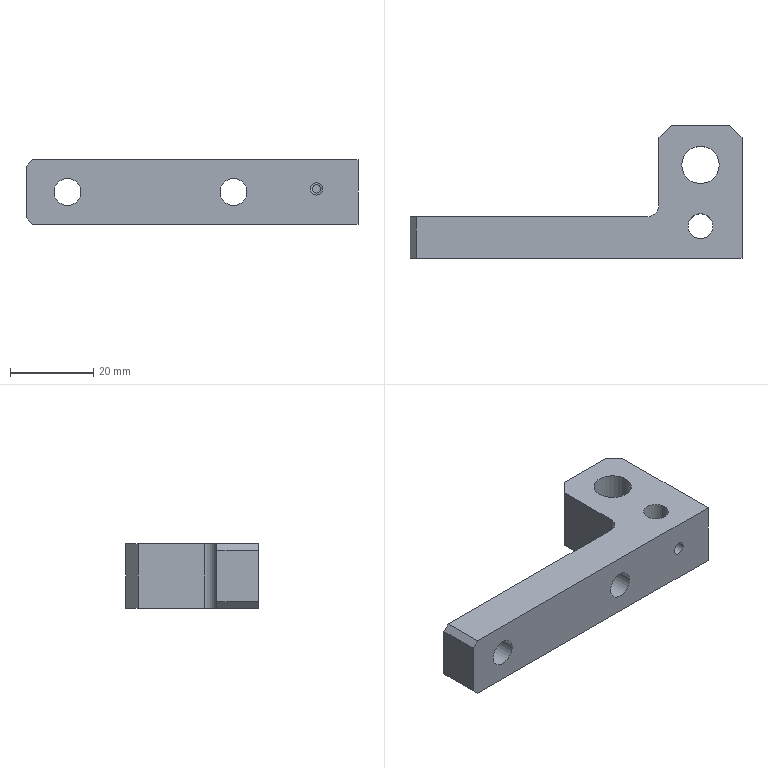NC program | NX | posted with a generic post | part box 80 x 32 x 15.5 mm
Lines 1772 to 1848 of 1848:
(PLANAR_MILL_3 , TOOL : D63面刀)
N3542 T10 M6
N3544 G54
N3546 G17 G0 G90 X74.5 Y2.5 B0. C0. S1600 M3
N3548 G43 Z20. H10
N3550 Z3.
N3552 G94 G1 Z0. F600.
N3554 X40.
N3556 X-40.
N3558 X-74.5
N3560 Z3.
N3562 G0 Z20.
N3564 M5
(PLANAR_MILL_6 , TOOL : 倒角D4-90度)
N3566 T05 M6
N3568 G54
N3570 G17 G0 G90 X-40. Y19.5 B0. C0. S3000 M3
N3572 G43 Z20. H5
N3574 Z1.5
N3576 G94 G1 Z-1.5 F800.
N3578 G41 Y17.5 D5
N3580 X40.
N3582 G2 X41.5 Y16. R1.5
N3584 G1 Y6.
N3586 G2 X40. Y4.5 R1.5
N3588 G1 X-17.
N3590 G3 X-18.5 Y3. R1.5
N3592 G1 Y-13.
N3594 G2 X-18.939 Y-14.061 R1.5
N3596 G1 X-21.939 Y-17.061
N3598 G2 X-23. Y-17.5 R1.5
N3600 G1 X-37.
N3602 G2 X-38.061 Y-17.061 R1.5
N3604 G1 X-41.061 Y-14.061
N3606 G2 X-41.5 Y-13. R1.5
N3608 G1 Y16.
N3610 G2 X-40. Y17.5 R1.5
N3612 G40
N3614 G1 Y19.5
N3616 Z1.5
N3618 G0 Z20.
(PLANAR_MILL_6_COPY_1 , TOOL : 倒角D4-90度)
N3620 X-30.119 Y7.924
N3622 Z0.5
N3624 G1 Z-1.5
N3626 G41 X-29.134 Y7.75
N3628 X-29.
N3630 G3 X-28.5 Y8.25 R0.5
N3632 X-30. Y9.75 R1.5
N3634 X-28.5 Y8.25 R-1.5
N3636 X-29. Y8.75 R0.5
N3638 G1 X-29.134
N3640 G40
N3642 X-30.119 Y8.576
N3644 Z0.5
N3646 G0 Z20.
N3648 X-28.535 Y-6.826
N3650 Z0.5
N3652 G1 Z-1.5
N3654 G41 X-27.551 Y-7.
N3656 X-27.5
N3658 G3 X-27. Y-6.5 R0.5
N3660 X-30. Y-3.5 R3.
N3662 X-27. Y-6.5 R-3.
N3664 X-27.551 Y-6. R0.503
N3666 G40
N3668 G1 X-28.535 Y-6.174
N3670 Z0.5
N3672 G0 Z20.
N3674 M5
N3676 M2